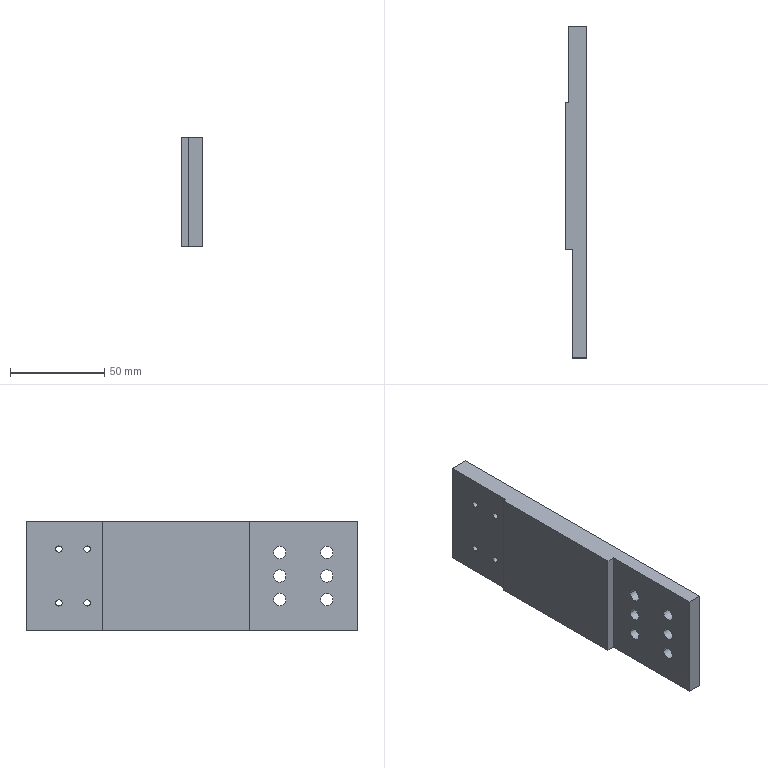Part | STEP file | ASND-0110-TPIM-064 | 1 solid | 42 faces | box 11.6 x 176 x 58 mm | volume 99143 mm3 | cylinder 28 | plane 14 | commonest cylinder face diameters 6.5 x20 3.4 x8